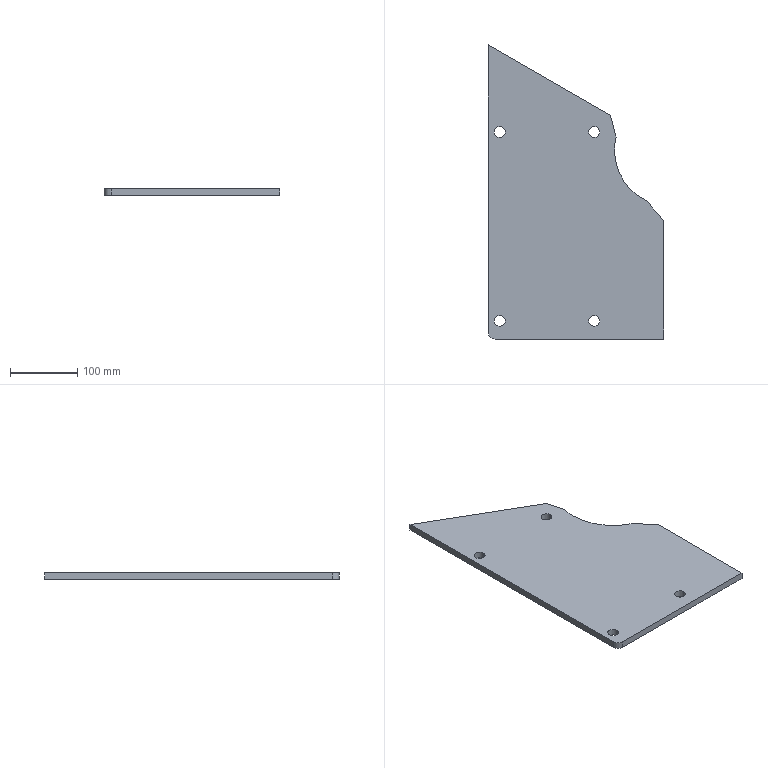Part | SolidWorks | features Extrusion 1, Fillet 1, HoleWzd 1 | 1 solid | 19 faces | box 260 x 436 x 10 mm | volume 861786 mm3 | cylinder 11 | plane 8 | commonest cylinder face diameters 16 x8 166 x2 20 x1
STEP:
#1=CARTESIAN_POINT('',(25.,27.,-5.));
#2=VERTEX_POINT('',#1);
#3=CARTESIAN_POINT('',(9.,27.,-5.));
#4=VERTEX_POINT('',#3);
#5=CARTESIAN_POINT('',(17.,27.,-5.));
#6=DIRECTION('',(0.,0.,-1.));
#7=DIRECTION('',(-1.,0.,0.));
#8=AXIS2_PLACEMENT_3D('',#5,#6,#7);
#9=CIRCLE('',#8,8.);
#10=EDGE_CURVE('',#2,#4,#9,.T.);
#11=ORIENTED_EDGE('',*,*,#10,.T.);
#12=CARTESIAN_POINT('',(9.,27.,5.));
#13=VERTEX_POINT('',#12);
#14=CARTESIAN_POINT('',(9.,27.,5.));
#15=DIRECTION('',(0.,0.,1.));
#16=VECTOR('',#15,1000.);
#17=LINE('',#14,#16);
#18=EDGE_CURVE('',#4,#13,#17,.T.);
#19=ORIENTED_EDGE('',*,*,#18,.T.);
#20=CARTESIAN_POINT('',(25.,27.,5.));
#21=VERTEX_POINT('',#20);
#22=CARTESIAN_POINT('',(17.,27.,5.));
#23=DIRECTION('',(0.,0.,1.));
#24=DIRECTION('',(1.,0.,0.));
#25=AXIS2_PLACEMENT_3D('',#22,#23,#24);
#26=CIRCLE('',#25,8.);
#27=EDGE_CURVE('',#13,#21,#26,.T.);
#28=ORIENTED_EDGE('',*,*,#27,.T.);
#29=CARTESIAN_POINT('',(25.,27.,5.));
#30=DIRECTION('',(0.,0.,1.));
#31=VECTOR('',#30,1000.);
#32=LINE('',#29,#31);
#33=EDGE_CURVE('',#2,#21,#32,.T.);
#34=ORIENTED_EDGE('',*,*,#33,.F.);
#35=EDGE_LOOP('',(#11,#19,#28,#34));
#36=FACE_OUTER_BOUND('',#35,.T.);
#37=CARTESIAN_POINT('',(17.,27.,5.));
#38=DIRECTION('',(0.,0.,1.));
#39=DIRECTION('',(1.,0.,0.));
#40=AXIS2_PLACEMENT_3D('',#37,#38,#39);
#41=CYLINDRICAL_SURFACE('',#40,8.);
#42=ADVANCED_FACE('',(#36),#41,.F.);
#43=CARTESIAN_POINT('',(165.,27.,-5.));
#44=VERTEX_POINT('',#43);
#45=CARTESIAN_POINT('',(149.,27.,-5.));
#46=VERTEX_POINT('',#45);
#47=CARTESIAN_POINT('',(157.,27.,-5.));
#48=DIRECTION('',(0.,0.,-1.));
#49=DIRECTION('',(-1.,0.,0.));
#50=AXIS2_PLACEMENT_3D('',#47,#48,#49);
#51=CIRCLE('',#50,8.);
#52=EDGE_CURVE('',#44,#46,#51,.T.);
#53=ORIENTED_EDGE('',*,*,#52,.T.);
#54=CARTESIAN_POINT('',(149.,27.,5.));
#55=VERTEX_POINT('',#54);
#56=CARTESIAN_POINT('',(149.,27.,5.));
#57=DIRECTION('',(0.,0.,1.));
#58=VECTOR('',#57,1000.);
#59=LINE('',#56,#58);
#60=EDGE_CURVE('',#46,#55,#59,.T.);
#61=ORIENTED_EDGE('',*,*,#60,.T.);
#62=CARTESIAN_POINT('',(165.,27.,5.));
#63=VERTEX_POINT('',#62);
#64=CARTESIAN_POINT('',(157.,27.,5.));
#65=DIRECTION('',(0.,0.,1.));
#66=DIRECTION('',(1.,0.,0.));
#67=AXIS2_PLACEMENT_3D('',#64,#65,#66);
#68=CIRCLE('',#67,8.);
#69=EDGE_CURVE('',#55,#63,#68,.T.);
#70=ORIENTED_EDGE('',*,*,#69,.T.);
#71=CARTESIAN_POINT('',(165.,27.,5.));
#72=DIRECTION('',(0.,0.,1.));
#73=VECTOR('',#72,1000.);
#74=LINE('',#71,#73);
#75=EDGE_CURVE('',#44,#63,#74,.T.);
#76=ORIENTED_EDGE('',*,*,#75,.F.);
#77=EDGE_LOOP('',(#53,#61,#70,#76));
#78=FACE_OUTER_BOUND('',#77,.T.);
#79=CARTESIAN_POINT('',(157.,27.,5.));
#80=DIRECTION('',(0.,0.,1.));
#81=DIRECTION('',(1.,0.,0.));
#82=AXIS2_PLACEMENT_3D('',#79,#80,#81);
#83=CYLINDRICAL_SURFACE('',#82,8.);
#84=ADVANCED_FACE('',(#78),#83,.F.);
#85=CARTESIAN_POINT('',(165.,307.,-5.));
#86=VERTEX_POINT('',#85);
#87=CARTESIAN_POINT('',(149.,307.,-5.));
#88=VERTEX_POINT('',#87);
#89=CARTESIAN_POINT('',(157.,307.,-5.));
#90=DIRECTION('',(0.,0.,-1.));
#91=DIRECTION('',(-1.,0.,0.));
#92=AXIS2_PLACEMENT_3D('',#89,#90,#91);
#93=CIRCLE('',#92,8.);
#94=EDGE_CURVE('',#86,#88,#93,.T.);
#95=ORIENTED_EDGE('',*,*,#94,.T.);
#96=CARTESIAN_POINT('',(149.,307.,5.));
#97=VERTEX_POINT('',#96);
#98=CARTESIAN_POINT('',(149.,307.,5.));
#99=DIRECTION('',(0.,0.,1.));
#100=VECTOR('',#99,1000.);
#101=LINE('',#98,#100);
#102=EDGE_CURVE('',#88,#97,#101,.T.);
#103=ORIENTED_EDGE('',*,*,#102,.T.);
#104=CARTESIAN_POINT('',(165.,307.,5.));
#105=VERTEX_POINT('',#104);
#106=CARTESIAN_POINT('',(157.,307.,5.));
#107=DIRECTION('',(0.,0.,1.));
#108=DIRECTION('',(1.,0.,0.));
#109=AXIS2_PLACEMENT_3D('',#106,#107,#108);
#110=CIRCLE('',#109,8.);
#111=EDGE_CURVE('',#97,#105,#110,.T.);
#112=ORIENTED_EDGE('',*,*,#111,.T.);
#113=CARTESIAN_POINT('',(165.,307.,5.));
#114=DIRECTION('',(0.,0.,1.));
#115=VECTOR('',#114,1000.);
#116=LINE('',#113,#115);
#117=EDGE_CURVE('',#86,#105,#116,.T.);
#118=ORIENTED_EDGE('',*,*,#117,.F.);
#119=EDGE_LOOP('',(#95,#103,#112,#118));
#120=FACE_OUTER_BOUND('',#119,.T.);
#121=CARTESIAN_POINT('',(157.,307.,5.));
#122=DIRECTION('',(0.,0.,1.));
#123=DIRECTION('',(1.,0.,0.));
#124=AXIS2_PLACEMENT_3D('',#121,#122,#123);
#125=CYLINDRICAL_SURFACE('',#124,8.);
#126=ADVANCED_FACE('',(#120),#125,.F.);
#127=CARTESIAN_POINT('',(25.,307.,-5.));
#128=VERTEX_POINT('',#127);
#129=CARTESIAN_POINT('',(9.,307.,-5.));
#130=VERTEX_POINT('',#129);
#131=CARTESIAN_POINT('',(17.,307.,-5.));
#132=DIRECTION('',(0.,0.,-1.));
#133=DIRECTION('',(-1.,0.,0.));
#134=AXIS2_PLACEMENT_3D('',#131,#132,#133);
#135=CIRCLE('',#134,8.);
#136=EDGE_CURVE('',#128,#130,#135,.T.);
#137=ORIENTED_EDGE('',*,*,#136,.T.);
#138=CARTESIAN_POINT('',(9.,307.,5.));
#139=VERTEX_POINT('',#138);
#140=CARTESIAN_POINT('',(9.,307.,5.));
#141=DIRECTION('',(0.,0.,1.));
#142=VECTOR('',#141,1000.);
#143=LINE('',#140,#142);
#144=EDGE_CURVE('',#130,#139,#143,.T.);
#145=ORIENTED_EDGE('',*,*,#144,.T.);
#146=CARTESIAN_POINT('',(25.,307.,5.));
#147=VERTEX_POINT('',#146);
#148=CARTESIAN_POINT('',(17.,307.,5.));
#149=DIRECTION('',(0.,0.,1.));
#150=DIRECTION('',(1.,0.,0.));
#151=AXIS2_PLACEMENT_3D('',#148,#149,#150);
#152=CIRCLE('',#151,8.);
#153=EDGE_CURVE('',#139,#147,#152,.T.);
#154=ORIENTED_EDGE('',*,*,#153,.T.);
#155=CARTESIAN_POINT('',(25.,307.,5.));
#156=DIRECTION('',(0.,0.,1.));
#157=VECTOR('',#156,1000.);
#158=LINE('',#155,#157);
#159=EDGE_CURVE('',#128,#147,#158,.T.);
#160=ORIENTED_EDGE('',*,*,#159,.F.);
#161=EDGE_LOOP('',(#137,#145,#154,#160));
#162=FACE_OUTER_BOUND('',#161,.T.);
#163=CARTESIAN_POINT('',(17.,307.,5.));
#164=DIRECTION('',(0.,0.,1.));
#165=DIRECTION('',(1.,0.,0.));
#166=AXIS2_PLACEMENT_3D('',#163,#164,#165);
#167=CYLINDRICAL_SURFACE('',#166,8.);
#168=ADVANCED_FACE('',(#162),#167,.F.);
#169=CARTESIAN_POINT('',(187.,280.,5.));
#170=VERTEX_POINT('',#169);
#171=CARTESIAN_POINT('',(189.323,299.5,5.));
#172=VERTEX_POINT('',#171);
#173=CARTESIAN_POINT('',(270.,280.,5.));
#174=DIRECTION('',(0.,0.,-1.));
#175=DIRECTION('',(-1.,0.,0.));
#176=AXIS2_PLACEMENT_3D('',#173,#174,#175);
#177=CIRCLE('',#176,83.);
#178=EDGE_CURVE('',#170,#172,#177,.T.);
#179=ORIENTED_EDGE('',*,*,#178,.F.);
#180=CARTESIAN_POINT('',(187.,280.,-5.));
#181=VERTEX_POINT('',#180);
#182=CARTESIAN_POINT('',(187.,280.,5.));
#183=DIRECTION('',(0.,0.,-1.));
#184=VECTOR('',#183,1000.);
#185=LINE('',#182,#184);
#186=EDGE_CURVE('',#170,#181,#185,.T.);
#187=ORIENTED_EDGE('',*,*,#186,.T.);
#188=CARTESIAN_POINT('',(189.323,299.5,-5.));
#189=VERTEX_POINT('',#188);
#190=CARTESIAN_POINT('',(270.,280.,-5.));
#191=DIRECTION('',(0.,0.,-1.));
#192=DIRECTION('',(-1.,0.,0.));
#193=AXIS2_PLACEMENT_3D('',#190,#191,#192);
#194=CIRCLE('',#193,83.);
#195=EDGE_CURVE('',#181,#189,#194,.T.);
#196=ORIENTED_EDGE('',*,*,#195,.T.);
#197=CARTESIAN_POINT('',(189.323,299.5,5.));
#198=DIRECTION('',(0.,0.,-1.));
#199=VECTOR('',#198,1000.);
#200=LINE('',#197,#199);
#201=EDGE_CURVE('',#172,#189,#200,.T.);
#202=ORIENTED_EDGE('',*,*,#201,.F.);
#203=EDGE_LOOP('',(#179,#187,#196,#202));
#204=FACE_OUTER_BOUND('',#203,.T.);
#205=CARTESIAN_POINT('',(270.,280.,5.));
#206=DIRECTION('',(0.,0.,-1.));
#207=DIRECTION('',(-1.,0.,0.));
#208=AXIS2_PLACEMENT_3D('',#205,#206,#207);
#209=CYLINDRICAL_SURFACE('',#208,83.);
#210=ADVANCED_FACE('',(#204),#209,.F.);
#211=CARTESIAN_POINT('',(157.,307.,5.));
#212=DIRECTION('',(0.,0.,1.));
#213=DIRECTION('',(1.,0.,0.));
#214=AXIS2_PLACEMENT_3D('',#211,#212,#213);
#215=CIRCLE('',#214,8.);
#216=EDGE_CURVE('',#105,#97,#215,.T.);
#217=ORIENTED_EDGE('',*,*,#216,.F.);
#218=ORIENTED_EDGE('',*,*,#111,.F.);
#219=EDGE_LOOP('',(#217,#218));
#220=FACE_BOUND('',#219,.T.);
#221=CARTESIAN_POINT('',(17.,307.,5.));
#222=DIRECTION('',(0.,0.,1.));
#223=DIRECTION('',(1.,0.,0.));
#224=AXIS2_PLACEMENT_3D('',#221,#222,#223);
#225=CIRCLE('',#224,8.);
#226=EDGE_CURVE('',#147,#139,#225,.T.);
#227=ORIENTED_EDGE('',*,*,#226,.F.);
#228=ORIENTED_EDGE('',*,*,#153,.F.);
#229=EDGE_LOOP('',(#227,#228));
#230=FACE_BOUND('',#229,.T.);
#231=CARTESIAN_POINT('',(0.,436.,5.));
#232=VERTEX_POINT('',#231);
#233=CARTESIAN_POINT('',(0.,10.,5.));
#234=VERTEX_POINT('',#233);
#235=CARTESIAN_POINT('',(0.,0.,5.));
#236=DIRECTION('',(0.,-1.,0.));
#237=VECTOR('',#236,1000.);
#238=LINE('',#235,#237);
#239=EDGE_CURVE('',#232,#234,#238,.T.);
#240=ORIENTED_EDGE('',*,*,#239,.T.);
#241=CARTESIAN_POINT('',(10.,0.,5.));
#242=VERTEX_POINT('',#241);
#243=CARTESIAN_POINT('',(10.,10.,5.));
#244=DIRECTION('',(0.,0.,1.));
#245=DIRECTION('',(-1.,0.,0.));
#246=AXIS2_PLACEMENT_3D('',#243,#244,#245);
#247=CIRCLE('',#246,10.);
#248=EDGE_CURVE('',#234,#242,#247,.T.);
#249=ORIENTED_EDGE('',*,*,#248,.T.);
#250=CARTESIAN_POINT('',(260.,0.,5.));
#251=VERTEX_POINT('',#250);
#252=CARTESIAN_POINT('',(0.,0.,5.));
#253=DIRECTION('',(1.,0.,0.));
#254=VECTOR('',#253,1000.);
#255=LINE('',#252,#254);
#256=EDGE_CURVE('',#242,#251,#255,.T.);
#257=ORIENTED_EDGE('',*,*,#256,.T.);
#258=CARTESIAN_POINT('',(260.,176.,5.));
#259=VERTEX_POINT('',#258);
#260=CARTESIAN_POINT('',(260.,0.,5.));
#261=DIRECTION('',(0.,1.,0.));
#262=VECTOR('',#261,1000.);
#263=LINE('',#260,#262);
#264=EDGE_CURVE('',#251,#259,#263,.T.);
#265=ORIENTED_EDGE('',*,*,#264,.T.);
#266=CARTESIAN_POINT('',(234.447,205.,5.));
#267=VERTEX_POINT('',#266);
#268=CARTESIAN_POINT('',(260.,176.,5.));
#269=DIRECTION('',(-0.6611,0.7503,0.));
#270=VECTOR('',#269,1000.);
#271=LINE('',#268,#270);
#272=EDGE_CURVE('',#259,#267,#271,.T.);
#273=ORIENTED_EDGE('',*,*,#272,.T.);
#274=CARTESIAN_POINT('',(270.,280.,5.));
#275=DIRECTION('',(0.,0.,-1.));
#276=DIRECTION('',(-1.,0.,0.));
#277=AXIS2_PLACEMENT_3D('',#274,#275,#276);
#278=CIRCLE('',#277,83.);
#279=EDGE_CURVE('',#267,#170,#278,.T.);
#280=ORIENTED_EDGE('',*,*,#279,.T.);
#281=ORIENTED_EDGE('',*,*,#178,.T.);
#282=CARTESIAN_POINT('',(181.,331.5,5.));
#283=VERTEX_POINT('',#282);
#284=CARTESIAN_POINT('',(181.,331.5,5.));
#285=DIRECTION('',(-0.2517,0.9678,0.));
#286=VECTOR('',#285,1000.);
#287=LINE('',#284,#286);
#288=EDGE_CURVE('',#172,#283,#287,.T.);
#289=ORIENTED_EDGE('',*,*,#288,.T.);
#290=CARTESIAN_POINT('',(0.,436.,5.));
#291=DIRECTION('',(-0.866,0.5,0.));
#292=VECTOR('',#291,1000.);
#293=LINE('',#290,#292);
#294=EDGE_CURVE('',#283,#232,#293,.T.);
#295=ORIENTED_EDGE('',*,*,#294,.T.);
#296=EDGE_LOOP('',(#240,#249,#257,#265,#273,#280,#281,#289,#295));
#297=FACE_OUTER_BOUND('',#296,.T.);
#298=CARTESIAN_POINT('',(157.,27.,5.));
#299=DIRECTION('',(0.,0.,1.));
#300=DIRECTION('',(1.,0.,0.));
#301=AXIS2_PLACEMENT_3D('',#298,#299,#300);
#302=CIRCLE('',#301,8.);
#303=EDGE_CURVE('',#63,#55,#302,.T.);
#304=ORIENTED_EDGE('',*,*,#303,.F.);
#305=ORIENTED_EDGE('',*,*,#69,.F.);
#306=EDGE_LOOP('',(#304,#305));
#307=FACE_BOUND('',#306,.T.);
#308=CARTESIAN_POINT('',(17.,27.,5.));
#309=DIRECTION('',(0.,0.,1.));
#310=DIRECTION('',(1.,0.,0.));
#311=AXIS2_PLACEMENT_3D('',#308,#309,#310);
#312=CIRCLE('',#311,8.);
#313=EDGE_CURVE('',#21,#13,#312,.T.);
#314=ORIENTED_EDGE('',*,*,#313,.F.);
#315=ORIENTED_EDGE('',*,*,#27,.F.);
#316=EDGE_LOOP('',(#314,#315));
#317=FACE_BOUND('',#316,.T.);
#318=CARTESIAN_POINT('',(270.,280.,5.));
#319=DIRECTION('',(0.,0.,-1.));
#320=DIRECTION('',(-1.,0.,0.));
#321=AXIS2_PLACEMENT_3D('',#318,#319,#320);
#322=PLANE('',#321);
#323=ADVANCED_FACE('',(#220,#230,#297,#307,#317),#322,.F.);
#324=ORIENTED_EDGE('',*,*,#256,.F.);
#325=CARTESIAN_POINT('',(10.,0.,-5.));
#326=VERTEX_POINT('',#325);
#327=CARTESIAN_POINT('',(10.,0.,5.));
#328=DIRECTION('',(0.,0.,-1.));
#329=VECTOR('',#328,1000.);
#330=LINE('',#327,#329);
#331=EDGE_CURVE('',#242,#326,#330,.T.);
#332=ORIENTED_EDGE('',*,*,#331,.T.);
#333=CARTESIAN_POINT('',(260.,0.,-5.));
#334=VERTEX_POINT('',#333);
#335=CARTESIAN_POINT('',(0.,0.,-5.));
#336=DIRECTION('',(1.,0.,0.));
#337=VECTOR('',#336,1000.);
#338=LINE('',#335,#337);
#339=EDGE_CURVE('',#326,#334,#338,.T.);
#340=ORIENTED_EDGE('',*,*,#339,.T.);
#341=CARTESIAN_POINT('',(260.,0.,5.));
#342=DIRECTION('',(0.,0.,-1.));
#343=VECTOR('',#342,1000.);
#344=LINE('',#341,#343);
#345=EDGE_CURVE('',#251,#334,#344,.T.);
#346=ORIENTED_EDGE('',*,*,#345,.F.);
#347=EDGE_LOOP('',(#324,#332,#340,#346));
#348=FACE_OUTER_BOUND('',#347,.T.);
#349=CARTESIAN_POINT('',(0.,0.,5.));
#350=DIRECTION('',(0.,1.,0.));
#351=DIRECTION('',(0.,0.,1.));
#352=AXIS2_PLACEMENT_3D('',#349,#350,#351);
#353=PLANE('',#352);
#354=ADVANCED_FACE('',(#348),#353,.F.);
#355=CARTESIAN_POINT('',(260.,176.,-5.));
#356=VERTEX_POINT('',#355);
#357=CARTESIAN_POINT('',(260.,0.,-5.));
#358=DIRECTION('',(0.,1.,0.));
#359=VECTOR('',#358,1000.);
#360=LINE('',#357,#359);
#361=EDGE_CURVE('',#334,#356,#360,.T.);
#362=ORIENTED_EDGE('',*,*,#361,.T.);
#363=CARTESIAN_POINT('',(260.,176.,5.));
#364=DIRECTION('',(0.,0.,-1.));
#365=VECTOR('',#364,1000.);
#366=LINE('',#363,#365);
#367=EDGE_CURVE('',#259,#356,#366,.T.);
#368=ORIENTED_EDGE('',*,*,#367,.F.);
#369=ORIENTED_EDGE('',*,*,#264,.F.);
#370=ORIENTED_EDGE('',*,*,#345,.T.);
#371=EDGE_LOOP('',(#362,#368,#369,#370));
#372=FACE_OUTER_BOUND('',#371,.T.);
#373=CARTESIAN_POINT('',(260.,0.,5.));
#374=DIRECTION('',(-1.,0.,0.));
#375=DIRECTION('',(0.,0.,1.));
#376=AXIS2_PLACEMENT_3D('',#373,#374,#375);
#377=PLANE('',#376);
#378=ADVANCED_FACE('',(#372),#377,.F.);
#379=CARTESIAN_POINT('',(234.447,205.,-5.));
#380=VERTEX_POINT('',#379);
#381=CARTESIAN_POINT('',(260.,176.,-5.));
#382=DIRECTION('',(-0.6611,0.7503,0.));
#383=VECTOR('',#382,1000.);
#384=LINE('',#381,#383);
#385=EDGE_CURVE('',#356,#380,#384,.T.);
#386=ORIENTED_EDGE('',*,*,#385,.T.);
#387=CARTESIAN_POINT('',(234.447,205.,5.));
#388=DIRECTION('',(0.,0.,-1.));
#389=VECTOR('',#388,1000.);
#390=LINE('',#387,#389);
#391=EDGE_CURVE('',#267,#380,#390,.T.);
#392=ORIENTED_EDGE('',*,*,#391,.F.);
#393=ORIENTED_EDGE('',*,*,#272,.F.);
#394=ORIENTED_EDGE('',*,*,#367,.T.);
#395=EDGE_LOOP('',(#386,#392,#393,#394));
#396=FACE_OUTER_BOUND('',#395,.T.);
#397=CARTESIAN_POINT('',(260.,176.,5.));
#398=DIRECTION('',(-0.7503,-0.6611,0.));
#399=DIRECTION('',(0.6611,-0.7503,0.));
#400=AXIS2_PLACEMENT_3D('',#397,#398,#399);
#401=PLANE('',#400);
#402=ADVANCED_FACE('',(#396),#401,.F.);
#403=ORIENTED_EDGE('',*,*,#186,.F.);
#404=ORIENTED_EDGE('',*,*,#279,.F.);
#405=ORIENTED_EDGE('',*,*,#391,.T.);
#406=CARTESIAN_POINT('',(270.,280.,-5.));
#407=DIRECTION('',(0.,0.,-1.));
#408=DIRECTION('',(-1.,0.,0.));
#409=AXIS2_PLACEMENT_3D('',#406,#407,#408);
#410=CIRCLE('',#409,83.);
#411=EDGE_CURVE('',#380,#181,#410,.T.);
#412=ORIENTED_EDGE('',*,*,#411,.T.);
#413=EDGE_LOOP('',(#403,#404,#405,#412));
#414=FACE_OUTER_BOUND('',#413,.T.);
#415=CARTESIAN_POINT('',(270.,280.,5.));
#416=DIRECTION('',(0.,0.,-1.));
#417=DIRECTION('',(-1.,0.,0.));
#418=AXIS2_PLACEMENT_3D('',#415,#416,#417);
#419=CYLINDRICAL_SURFACE('',#418,83.);
#420=ADVANCED_FACE('',(#414),#419,.F.);
#421=CARTESIAN_POINT('',(181.,331.5,-5.));
#422=VERTEX_POINT('',#421);
#423=CARTESIAN_POINT('',(181.,331.5,-5.));
#424=DIRECTION('',(-0.2517,0.9678,0.));
#425=VECTOR('',#424,1000.);
#426=LINE('',#423,#425);
#427=EDGE_CURVE('',#189,#422,#426,.T.);
#428=ORIENTED_EDGE('',*,*,#427,.T.);
#429=CARTESIAN_POINT('',(181.,331.5,5.));
#430=DIRECTION('',(0.,0.,-1.));
#431=VECTOR('',#430,1000.);
#432=LINE('',#429,#431);
#433=EDGE_CURVE('',#283,#422,#432,.T.);
#434=ORIENTED_EDGE('',*,*,#433,.F.);
#435=ORIENTED_EDGE('',*,*,#288,.F.);
#436=ORIENTED_EDGE('',*,*,#201,.T.);
#437=EDGE_LOOP('',(#428,#434,#435,#436));
#438=FACE_OUTER_BOUND('',#437,.T.);
#439=CARTESIAN_POINT('',(181.,331.5,5.));
#440=DIRECTION('',(-0.9678,-0.2517,0.));
#441=DIRECTION('',(0.2517,-0.9678,0.));
#442=AXIS2_PLACEMENT_3D('',#439,#440,#441);
#443=PLANE('',#442);
#444=ADVANCED_FACE('',(#438),#443,.F.);
#445=CARTESIAN_POINT('',(0.,436.,-5.));
#446=VERTEX_POINT('',#445);
#447=CARTESIAN_POINT('',(0.,436.,-5.));
#448=DIRECTION('',(-0.866,0.5,0.));
#449=VECTOR('',#448,1000.);
#450=LINE('',#447,#449);
#451=EDGE_CURVE('',#422,#446,#450,.T.);
#452=ORIENTED_EDGE('',*,*,#451,.T.);
#453=CARTESIAN_POINT('',(0.,436.,5.));
#454=DIRECTION('',(0.,0.,-1.));
#455=VECTOR('',#454,1000.);
#456=LINE('',#453,#455);
#457=EDGE_CURVE('',#232,#446,#456,.T.);
#458=ORIENTED_EDGE('',*,*,#457,.F.);
#459=ORIENTED_EDGE('',*,*,#294,.F.);
#460=ORIENTED_EDGE('',*,*,#433,.T.);
#461=EDGE_LOOP('',(#452,#458,#459,#460));
#462=FACE_OUTER_BOUND('',#461,.T.);
#463=CARTESIAN_POINT('',(0.,436.,5.));
#464=DIRECTION('',(-0.5,-0.866,0.));
#465=DIRECTION('',(0.866,-0.5,0.));
#466=AXIS2_PLACEMENT_3D('',#463,#464,#465);
#467=PLANE('',#466);
#468=ADVANCED_FACE('',(#462),#467,.F.);
#469=CARTESIAN_POINT('',(0.,10.,-5.));
#470=VERTEX_POINT('',#469);
#471=CARTESIAN_POINT('',(0.,0.,-5.));
#472=DIRECTION('',(0.,-1.,0.));
#473=VECTOR('',#472,1000.);
#474=LINE('',#471,#473);
#475=EDGE_CURVE('',#446,#470,#474,.T.);
#476=ORIENTED_EDGE('',*,*,#475,.T.);
#477=CARTESIAN_POINT('',(0.,10.,5.));
#478=DIRECTION('',(0.,0.,1.));
#479=VECTOR('',#478,1000.);
#480=LINE('',#477,#479);
#481=EDGE_CURVE('',#470,#234,#480,.T.);
#482=ORIENTED_EDGE('',*,*,#481,.T.);
#483=ORIENTED_EDGE('',*,*,#239,.F.);
#484=ORIENTED_EDGE('',*,*,#457,.T.);
#485=EDGE_LOOP('',(#476,#482,#483,#484));
#486=FACE_OUTER_BOUND('',#485,.T.);
#487=CARTESIAN_POINT('',(0.,0.,5.));
#488=DIRECTION('',(1.,0.,0.));
#489=DIRECTION('',(0.,0.,-1.));
#490=AXIS2_PLACEMENT_3D('',#487,#488,#489);
#491=PLANE('',#490);
#492=ADVANCED_FACE('',(#486),#491,.F.);
#493=ORIENTED_EDGE('',*,*,#10,.F.);
#494=CARTESIAN_POINT('',(17.,27.,-5.));
#495=DIRECTION('',(0.,0.,-1.));
#496=DIRECTION('',(-1.,0.,0.));
#497=AXIS2_PLACEMENT_3D('',#494,#495,#496);
#498=CIRCLE('',#497,8.);
#499=EDGE_CURVE('',#4,#2,#498,.T.);
#500=ORIENTED_EDGE('',*,*,#499,.F.);
#501=EDGE_LOOP('',(#493,#500));
#502=FACE_BOUND('',#501,.T.);
#503=ORIENTED_EDGE('',*,*,#52,.F.);
#504=CARTESIAN_POINT('',(157.,27.,-5.));
#505=DIRECTION('',(0.,0.,-1.));
#506=DIRECTION('',(-1.,0.,0.));
#507=AXIS2_PLACEMENT_3D('',#504,#505,#506);
#508=CIRCLE('',#507,8.);
#509=EDGE_CURVE('',#46,#44,#508,.T.);
#510=ORIENTED_EDGE('',*,*,#509,.F.);
#511=EDGE_LOOP('',(#503,#510));
#512=FACE_BOUND('',#511,.T.);
#513=ORIENTED_EDGE('',*,*,#94,.F.);
#514=CARTESIAN_POINT('',(157.,307.,-5.));
#515=DIRECTION('',(0.,0.,-1.));
#516=DIRECTION('',(-1.,0.,0.));
#517=AXIS2_PLACEMENT_3D('',#514,#515,#516);
#518=CIRCLE('',#517,8.);
#519=EDGE_CURVE('',#88,#86,#518,.T.);
#520=ORIENTED_EDGE('',*,*,#519,.F.);
#521=EDGE_LOOP('',(#513,#520));
#522=FACE_BOUND('',#521,.T.);
#523=ORIENTED_EDGE('',*,*,#136,.F.);
#524=CARTESIAN_POINT('',(17.,307.,-5.));
#525=DIRECTION('',(0.,0.,-1.));
#526=DIRECTION('',(-1.,0.,0.));
#527=AXIS2_PLACEMENT_3D('',#524,#525,#526);
#528=CIRCLE('',#527,8.);
#529=EDGE_CURVE('',#130,#128,#528,.T.);
#530=ORIENTED_EDGE('',*,*,#529,.F.);
#531=EDGE_LOOP('',(#523,#530));
#532=FACE_BOUND('',#531,.T.);
#533=ORIENTED_EDGE('',*,*,#339,.F.);
#534=CARTESIAN_POINT('',(10.,10.,-5.));
#535=DIRECTION('',(0.,0.,-1.));
#536=DIRECTION('',(-1.,0.,0.));
#537=AXIS2_PLACEMENT_3D('',#534,#535,#536);
#538=CIRCLE('',#537,10.);
#539=EDGE_CURVE('',#326,#470,#538,.T.);
#540=ORIENTED_EDGE('',*,*,#539,.T.);
#541=ORIENTED_EDGE('',*,*,#475,.F.);
#542=ORIENTED_EDGE('',*,*,#451,.F.);
#543=ORIENTED_EDGE('',*,*,#427,.F.);
#544=ORIENTED_EDGE('',*,*,#195,.F.);
#545=ORIENTED_EDGE('',*,*,#411,.F.);
#546=ORIENTED_EDGE('',*,*,#385,.F.);
#547=ORIENTED_EDGE('',*,*,#361,.F.);
#548=EDGE_LOOP('',(#533,#540,#541,#542,#543,#544,#545,#546,#547));
#549=FACE_OUTER_BOUND('',#548,.T.);
#550=CARTESIAN_POINT('',(270.,280.,-5.));
#551=DIRECTION('',(0.,0.,-1.));
#552=DIRECTION('',(-1.,0.,0.));
#553=AXIS2_PLACEMENT_3D('',#550,#551,#552);
#554=PLANE('',#553);
#555=ADVANCED_FACE('',(#502,#512,#522,#532,#549),#554,.T.);
#556=ORIENTED_EDGE('',*,*,#144,.F.);
#557=ORIENTED_EDGE('',*,*,#529,.T.);
#558=ORIENTED_EDGE('',*,*,#159,.T.);
#559=ORIENTED_EDGE('',*,*,#226,.T.);
#560=EDGE_LOOP('',(#556,#557,#558,#559));
#561=FACE_OUTER_BOUND('',#560,.T.);
#562=CARTESIAN_POINT('',(17.,307.,5.));
#563=DIRECTION('',(0.,0.,1.));
#564=DIRECTION('',(1.,0.,0.));
#565=AXIS2_PLACEMENT_3D('',#562,#563,#564);
#566=CYLINDRICAL_SURFACE('',#565,8.);
#567=ADVANCED_FACE('',(#561),#566,.F.);
#568=ORIENTED_EDGE('',*,*,#102,.F.);
#569=ORIENTED_EDGE('',*,*,#519,.T.);
#570=ORIENTED_EDGE('',*,*,#117,.T.);
#571=ORIENTED_EDGE('',*,*,#216,.T.);
#572=EDGE_LOOP('',(#568,#569,#570,#571));
#573=FACE_OUTER_BOUND('',#572,.T.);
#574=CARTESIAN_POINT('',(157.,307.,5.));
#575=DIRECTION('',(0.,0.,1.));
#576=DIRECTION('',(1.,0.,0.));
#577=AXIS2_PLACEMENT_3D('',#574,#575,#576);
#578=CYLINDRICAL_SURFACE('',#577,8.);
#579=ADVANCED_FACE('',(#573),#578,.F.);
#580=ORIENTED_EDGE('',*,*,#60,.F.);
#581=ORIENTED_EDGE('',*,*,#509,.T.);
#582=ORIENTED_EDGE('',*,*,#75,.T.);
#583=ORIENTED_EDGE('',*,*,#303,.T.);
#584=EDGE_LOOP('',(#580,#581,#582,#583));
#585=FACE_OUTER_BOUND('',#584,.T.);
#586=CARTESIAN_POINT('',(157.,27.,5.));
#587=DIRECTION('',(0.,0.,1.));
#588=DIRECTION('',(1.,0.,0.));
#589=AXIS2_PLACEMENT_3D('',#586,#587,#588);
#590=CYLINDRICAL_SURFACE('',#589,8.);
#591=ADVANCED_FACE('',(#585),#590,.F.);
#592=ORIENTED_EDGE('',*,*,#18,.F.);
#593=ORIENTED_EDGE('',*,*,#499,.T.);
#594=ORIENTED_EDGE('',*,*,#33,.T.);
#595=ORIENTED_EDGE('',*,*,#313,.T.);
#596=EDGE_LOOP('',(#592,#593,#594,#595));
#597=FACE_OUTER_BOUND('',#596,.T.);
#598=CARTESIAN_POINT('',(17.,27.,5.));
#599=DIRECTION('',(0.,0.,1.));
#600=DIRECTION('',(1.,0.,0.));
#601=AXIS2_PLACEMENT_3D('',#598,#599,#600);
#602=CYLINDRICAL_SURFACE('',#601,8.);
#603=ADVANCED_FACE('',(#597),#602,.F.);
#604=ORIENTED_EDGE('',*,*,#248,.F.);
#605=ORIENTED_EDGE('',*,*,#481,.F.);
#606=ORIENTED_EDGE('',*,*,#539,.F.);
#607=ORIENTED_EDGE('',*,*,#331,.F.);
#608=EDGE_LOOP('',(#604,#605,#606,#607));
#609=FACE_OUTER_BOUND('',#608,.T.);
#610=CARTESIAN_POINT('',(10.,10.,5.));
#611=DIRECTION('',(0.,0.,-1.));
#612=DIRECTION('',(-1.,0.,0.));
#613=AXIS2_PLACEMENT_3D('',#610,#611,#612);
#614=CYLINDRICAL_SURFACE('',#613,10.);
#615=ADVANCED_FACE('',(#609),#614,.T.);
#616=CLOSED_SHELL('',(#42,#84,#126,#168,#210,#323,#354,#378,#402,#420,#444,#468,#492,#555,#567,#579,#591,#603,#615));
#617=MANIFOLD_SOLID_BREP('',#616);
#618=CARTESIAN_POINT('',(0.,0.,0.));
#619=DIRECTION('',(0.,0.,1.));
#620=DIRECTION('',(1.,0.,0.));
#621=AXIS2_PLACEMENT_3D('',#618,#619,#620);
#622=(LENGTH_UNIT()NAMED_UNIT(*)SI_UNIT(.MILLI.,.METRE.));
#623=UNCERTAINTY_MEASURE_WITH_UNIT(LENGTH_MEASURE(0.00001),#622,'','');
#624=(NAMED_UNIT(*)PLANE_ANGLE_UNIT()SI_UNIT($,.RADIAN.));
#625=(NAMED_UNIT(*)SI_UNIT($,.STERADIAN.)SOLID_ANGLE_UNIT());
#626=(GEOMETRIC_REPRESENTATION_CONTEXT(3)GLOBAL_UNCERTAINTY_ASSIGNED_CONTEXT((#623))GLOBAL_UNIT_ASSIGNED_CONTEXT((#622,#624,#625))REPRESENTATION_CONTEXT('',''));
#627=ADVANCED_BREP_SHAPE_REPRESENTATION('',(#617,#621),#626);